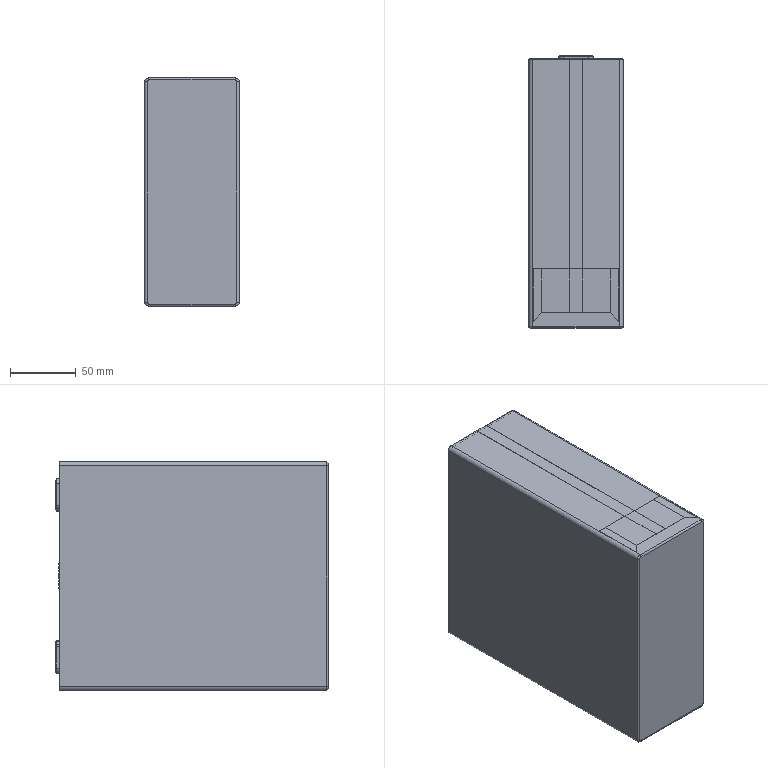Part | NX | features BREP 2 | 2 solids | 290 faces | box 71.65 x 206.8 x 174 mm | volume 2542557 mm3 | plane 193 | cylinder 82 | cone 11 | spline 4 | commonest cylinder face diameters 6 x20 2 x12 7.4 x6 8.4 x6 3.4 x4 4.2 x4